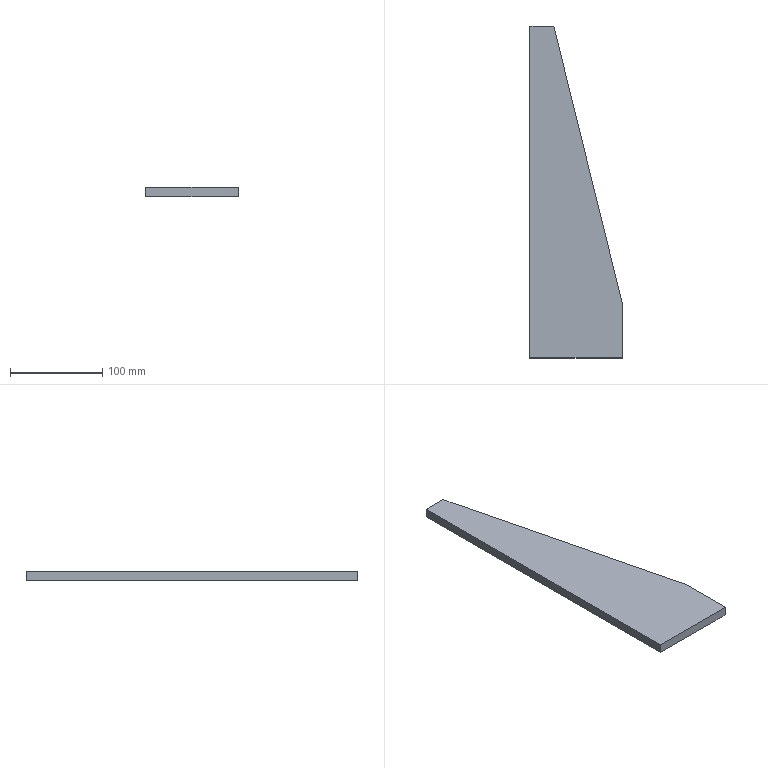Part | SolidWorks | features Extrusion 1 | 1 solid | 7 faces | box 100 x 360 x 10 mm | volume 249000 mm3 | plane 7
STEP:
#1=CARTESIAN_POINT('',(0.,360.,0.));
#2=VERTEX_POINT('',#1);
#3=CARTESIAN_POINT('',(0.,0.,0.));
#4=VERTEX_POINT('',#3);
#5=CARTESIAN_POINT('',(0.,360.,0.));
#6=DIRECTION('',(0.,-1.,0.));
#7=VECTOR('',#6,1000.);
#8=LINE('',#5,#7);
#9=EDGE_CURVE('',#2,#4,#8,.T.);
#10=ORIENTED_EDGE('',*,*,#9,.T.);
#11=CARTESIAN_POINT('',(0.,0.,10.));
#12=VERTEX_POINT('',#11);
#13=CARTESIAN_POINT('',(0.,0.,10.));
#14=DIRECTION('',(0.,0.,-1.));
#15=VECTOR('',#14,1000.);
#16=LINE('',#13,#15);
#17=EDGE_CURVE('',#12,#4,#16,.T.);
#18=ORIENTED_EDGE('',*,*,#17,.F.);
#19=CARTESIAN_POINT('',(0.,360.,10.));
#20=VERTEX_POINT('',#19);
#21=CARTESIAN_POINT('',(0.,360.,10.));
#22=DIRECTION('',(0.,-1.,0.));
#23=VECTOR('',#22,1000.);
#24=LINE('',#21,#23);
#25=EDGE_CURVE('',#20,#12,#24,.T.);
#26=ORIENTED_EDGE('',*,*,#25,.F.);
#27=CARTESIAN_POINT('',(0.,360.,10.));
#28=DIRECTION('',(0.,0.,-1.));
#29=VECTOR('',#28,1000.);
#30=LINE('',#27,#29);
#31=EDGE_CURVE('',#20,#2,#30,.T.);
#32=ORIENTED_EDGE('',*,*,#31,.T.);
#33=EDGE_LOOP('',(#10,#18,#26,#32));
#34=FACE_OUTER_BOUND('',#33,.T.);
#35=CARTESIAN_POINT('',(0.,360.,10.));
#36=DIRECTION('',(1.,0.,0.));
#37=DIRECTION('',(0.,1.,0.));
#38=AXIS2_PLACEMENT_3D('',#35,#36,#37);
#39=PLANE('',#38);
#40=ADVANCED_FACE('',(#34),#39,.F.);
#41=CARTESIAN_POINT('',(100.,0.,0.));
#42=VERTEX_POINT('',#41);
#43=CARTESIAN_POINT('',(0.,0.,0.));
#44=DIRECTION('',(1.,0.,0.));
#45=VECTOR('',#44,1000.);
#46=LINE('',#43,#45);
#47=EDGE_CURVE('',#4,#42,#46,.T.);
#48=ORIENTED_EDGE('',*,*,#47,.T.);
#49=CARTESIAN_POINT('',(100.,0.,10.));
#50=VERTEX_POINT('',#49);
#51=CARTESIAN_POINT('',(100.,0.,10.));
#52=DIRECTION('',(0.,0.,-1.));
#53=VECTOR('',#52,1000.);
#54=LINE('',#51,#53);
#55=EDGE_CURVE('',#50,#42,#54,.T.);
#56=ORIENTED_EDGE('',*,*,#55,.F.);
#57=CARTESIAN_POINT('',(0.,0.,10.));
#58=DIRECTION('',(1.,0.,0.));
#59=VECTOR('',#58,1000.);
#60=LINE('',#57,#59);
#61=EDGE_CURVE('',#12,#50,#60,.T.);
#62=ORIENTED_EDGE('',*,*,#61,.F.);
#63=ORIENTED_EDGE('',*,*,#17,.T.);
#64=EDGE_LOOP('',(#48,#56,#62,#63));
#65=FACE_OUTER_BOUND('',#64,.T.);
#66=CARTESIAN_POINT('',(0.,0.,10.));
#67=DIRECTION('',(0.,1.,0.));
#68=DIRECTION('',(0.,0.,1.));
#69=AXIS2_PLACEMENT_3D('',#66,#67,#68);
#70=PLANE('',#69);
#71=ADVANCED_FACE('',(#65),#70,.F.);
#72=CARTESIAN_POINT('',(100.,60.,0.));
#73=VERTEX_POINT('',#72);
#74=CARTESIAN_POINT('',(100.,0.,0.));
#75=DIRECTION('',(0.,1.,0.));
#76=VECTOR('',#75,1000.);
#77=LINE('',#74,#76);
#78=EDGE_CURVE('',#42,#73,#77,.T.);
#79=ORIENTED_EDGE('',*,*,#78,.T.);
#80=CARTESIAN_POINT('',(100.,60.,10.));
#81=VERTEX_POINT('',#80);
#82=CARTESIAN_POINT('',(100.,60.,10.));
#83=DIRECTION('',(0.,0.,-1.));
#84=VECTOR('',#83,1000.);
#85=LINE('',#82,#84);
#86=EDGE_CURVE('',#81,#73,#85,.T.);
#87=ORIENTED_EDGE('',*,*,#86,.F.);
#88=CARTESIAN_POINT('',(100.,0.,10.));
#89=DIRECTION('',(0.,1.,0.));
#90=VECTOR('',#89,1000.);
#91=LINE('',#88,#90);
#92=EDGE_CURVE('',#50,#81,#91,.T.);
#93=ORIENTED_EDGE('',*,*,#92,.F.);
#94=ORIENTED_EDGE('',*,*,#55,.T.);
#95=EDGE_LOOP('',(#79,#87,#93,#94));
#96=FACE_OUTER_BOUND('',#95,.T.);
#97=CARTESIAN_POINT('',(100.,0.,10.));
#98=DIRECTION('',(-1.,0.,0.));
#99=DIRECTION('',(0.,0.,1.));
#100=AXIS2_PLACEMENT_3D('',#97,#98,#99);
#101=PLANE('',#100);
#102=ADVANCED_FACE('',(#96),#101,.F.);
#103=CARTESIAN_POINT('',(26.,360.,0.));
#104=VERTEX_POINT('',#103);
#105=CARTESIAN_POINT('',(100.,60.,0.));
#106=DIRECTION('',(-0.2395,0.9709,0.));
#107=VECTOR('',#106,1000.);
#108=LINE('',#105,#107);
#109=EDGE_CURVE('',#73,#104,#108,.T.);
#110=ORIENTED_EDGE('',*,*,#109,.T.);
#111=CARTESIAN_POINT('',(26.,360.,10.));
#112=VERTEX_POINT('',#111);
#113=CARTESIAN_POINT('',(26.,360.,10.));
#114=DIRECTION('',(0.,0.,-1.));
#115=VECTOR('',#114,1000.);
#116=LINE('',#113,#115);
#117=EDGE_CURVE('',#112,#104,#116,.T.);
#118=ORIENTED_EDGE('',*,*,#117,.F.);
#119=CARTESIAN_POINT('',(100.,60.,10.));
#120=DIRECTION('',(-0.2395,0.9709,0.));
#121=VECTOR('',#120,1000.);
#122=LINE('',#119,#121);
#123=EDGE_CURVE('',#81,#112,#122,.T.);
#124=ORIENTED_EDGE('',*,*,#123,.F.);
#125=ORIENTED_EDGE('',*,*,#86,.T.);
#126=EDGE_LOOP('',(#110,#118,#124,#125));
#127=FACE_OUTER_BOUND('',#126,.T.);
#128=CARTESIAN_POINT('',(100.,60.,10.));
#129=DIRECTION('',(-0.9709,-0.2395,0.));
#130=DIRECTION('',(0.2395,-0.9709,0.));
#131=AXIS2_PLACEMENT_3D('',#128,#129,#130);
#132=PLANE('',#131);
#133=ADVANCED_FACE('',(#127),#132,.F.);
#134=CARTESIAN_POINT('',(26.,360.,0.));
#135=DIRECTION('',(-1.,0.,0.));
#136=VECTOR('',#135,1000.);
#137=LINE('',#134,#136);
#138=EDGE_CURVE('',#104,#2,#137,.T.);
#139=ORIENTED_EDGE('',*,*,#138,.T.);
#140=ORIENTED_EDGE('',*,*,#31,.F.);
#141=CARTESIAN_POINT('',(26.,360.,10.));
#142=DIRECTION('',(-1.,0.,0.));
#143=VECTOR('',#142,1000.);
#144=LINE('',#141,#143);
#145=EDGE_CURVE('',#112,#20,#144,.T.);
#146=ORIENTED_EDGE('',*,*,#145,.F.);
#147=ORIENTED_EDGE('',*,*,#117,.T.);
#148=EDGE_LOOP('',(#139,#140,#146,#147));
#149=FACE_OUTER_BOUND('',#148,.T.);
#150=CARTESIAN_POINT('',(26.,360.,10.));
#151=DIRECTION('',(0.,-1.,0.));
#152=DIRECTION('',(0.,0.,-1.));
#153=AXIS2_PLACEMENT_3D('',#150,#151,#152);
#154=PLANE('',#153);
#155=ADVANCED_FACE('',(#149),#154,.F.);
#156=ORIENTED_EDGE('',*,*,#25,.T.);
#157=ORIENTED_EDGE('',*,*,#61,.T.);
#158=ORIENTED_EDGE('',*,*,#92,.T.);
#159=ORIENTED_EDGE('',*,*,#123,.T.);
#160=ORIENTED_EDGE('',*,*,#145,.T.);
#161=EDGE_LOOP('',(#156,#157,#158,#159,#160));
#162=FACE_OUTER_BOUND('',#161,.T.);
#163=CARTESIAN_POINT('',(0.,0.,10.));
#164=DIRECTION('',(0.,0.,1.));
#165=DIRECTION('',(1.,0.,0.));
#166=AXIS2_PLACEMENT_3D('',#163,#164,#165);
#167=PLANE('',#166);
#168=ADVANCED_FACE('',(#162),#167,.T.);
#169=ORIENTED_EDGE('',*,*,#9,.F.);
#170=ORIENTED_EDGE('',*,*,#138,.F.);
#171=ORIENTED_EDGE('',*,*,#109,.F.);
#172=ORIENTED_EDGE('',*,*,#78,.F.);
#173=ORIENTED_EDGE('',*,*,#47,.F.);
#174=EDGE_LOOP('',(#169,#170,#171,#172,#173));
#175=FACE_OUTER_BOUND('',#174,.T.);
#176=CARTESIAN_POINT('',(0.,0.,0.));
#177=DIRECTION('',(0.,0.,1.));
#178=DIRECTION('',(1.,0.,0.));
#179=AXIS2_PLACEMENT_3D('',#176,#177,#178);
#180=PLANE('',#179);
#181=ADVANCED_FACE('',(#175),#180,.F.);
#182=CLOSED_SHELL('',(#40,#71,#102,#133,#155,#168,#181));
#183=MANIFOLD_SOLID_BREP('',#182);
#184=CARTESIAN_POINT('',(0.,0.,0.));
#185=DIRECTION('',(0.,0.,1.));
#186=DIRECTION('',(1.,0.,0.));
#187=AXIS2_PLACEMENT_3D('',#184,#185,#186);
#188=(LENGTH_UNIT()NAMED_UNIT(*)SI_UNIT(.MILLI.,.METRE.));
#189=UNCERTAINTY_MEASURE_WITH_UNIT(LENGTH_MEASURE(0.00001),#188,'','');
#190=(NAMED_UNIT(*)PLANE_ANGLE_UNIT()SI_UNIT($,.RADIAN.));
#191=(NAMED_UNIT(*)SI_UNIT($,.STERADIAN.)SOLID_ANGLE_UNIT());
#192=(GEOMETRIC_REPRESENTATION_CONTEXT(3)GLOBAL_UNCERTAINTY_ASSIGNED_CONTEXT((#189))GLOBAL_UNIT_ASSIGNED_CONTEXT((#188,#190,#191))REPRESENTATION_CONTEXT('',''));
#193=ADVANCED_BREP_SHAPE_REPRESENTATION('',(#183,#187),#192);